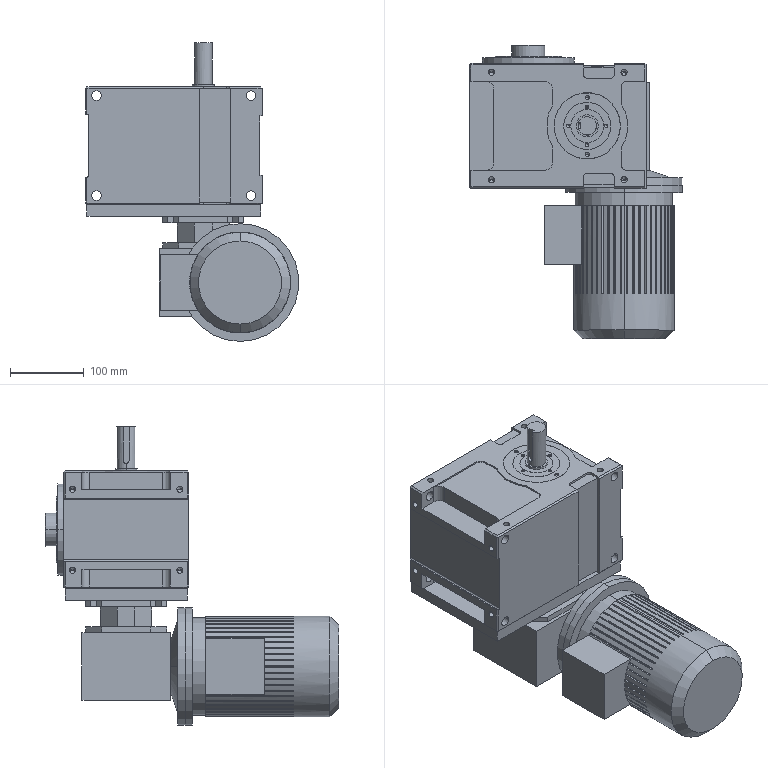Part | 6 solids | 837 faces | box 290 x 399 x 406 mm | volume 12134677 mm3 | plane 449 | cylinder 175 | spline 137 | cone 74 | torus 2 | commonest cylinder face diameters 8.5 x32 4.7 x16 13 x16 6.75 x12 10 x12 11 x12